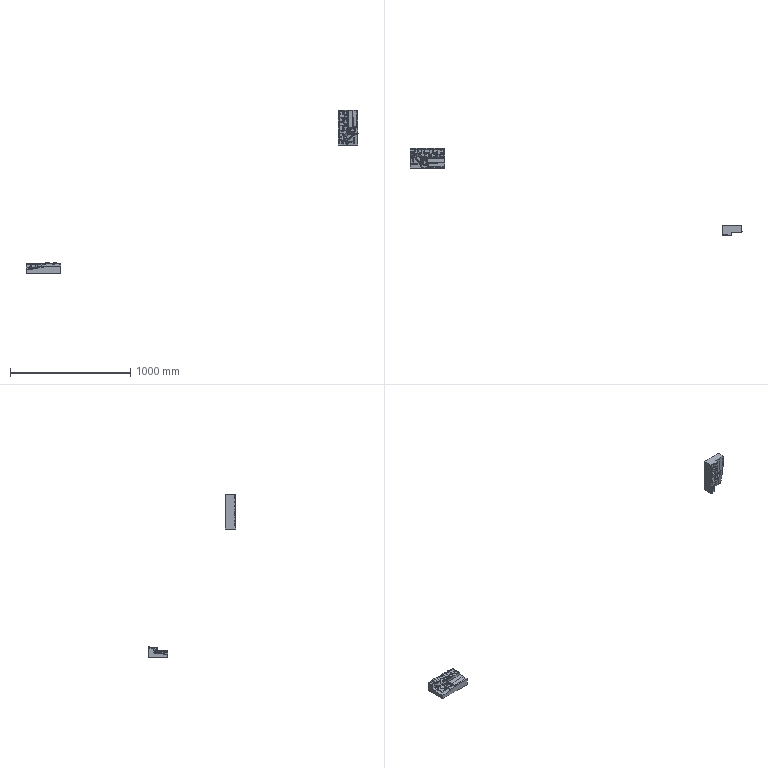NC program | NX | posted with a generic post | part box 2756 x 729.572 x 1353 mm
Lines 40259 to 41352 of 54396:
(CAVITY_MILL_1_COPY_COPY , TOOL : D6R3)
N80504 M6
N80506 G54
N80508 G17 G0 G90 X-104.537 Y-0.08 B0. C0. S3000 M3
N80510 G43 Z97. H0
N80512 Z88.216
N80514 G94 G1 Z88.016 F2500.
N80516 X-101.653 Y0.312
N80518 X-98.238 Y0.776
N80520 X-97.634 Y0.793
N80522 G2 X-96.274 Y0.137 R1.531
N80524 G1 X-96.255 Y-0.466
N80526 X-96.271 Y-7.828
N80528 G2 X-96.837 Y-8.503 R0.687
N80530 G1 X-97.634 Y-8.646
N80532 X-101.51 Y-8.335
N80534 X-104.477 Y-8.097
N80536 Z88.216
N80538 G0 Z89.3
N80540 X-104.765 Y2.482
N80542 Z88.019
N80544 G1 Z87.819
N80546 X-104.68 Y0.984
N80548 X-101.685 Y1.154
N80550 X-98.008 Y1.363
N80552 G2 X-95.577 Y0.741 R4.145
N80554 G1 X-95.179 Y0.137
N80556 X-95.167 Y-0.466
N80558 X-95.165 Y-7.707
N80560 X-95.217 Y-8.141
N80562 G2 X-97.029 Y-9.164 R2.101
N80564 X-101.54 Y-9.093 R116.617
N80566 G1 X-104.539 Y-8.987
N80568 X-104.627 Y-10.446
N80570 Z88.019
N80572 G0 Z88.316
N80574 X-104.659 Y3.
N80576 Z87.823
N80578 G1 Z87.623
N80580 X-104.604 Y1.515
N80582 X-101.605 Y1.598
N80584 G2 X-97.634 Y1.684 R323.824
N80586 X-95.101 Y1.023 R4.533
N80588 X-94.83 Y0.807 R1.373
N80590 G1 X-92.945 Y-1.138
N80592 Z87.823
N80594 G0 Z88.513
N80596 X-104.282 Y3.348
N80598 Z87.626
N80600 G1 Z87.426
N80602 X-104.24 Y1.858
N80604 X-101.24 Y1.924
N80606 G2 X-97.634 Y1.989 R469.677
N80608 X-95.269 Y1.542 R6.532
N80610 G1 X-92.399 Y0.42
N80612 Z87.626
N80614 G0 Z88.623
N80616 X-104.188 Y3.801
N80618 Z87.232
N80620 G1 Z87.032
N80622 X-104.165 Y2.309
N80624 X-101.166 Y2.34
N80626 G2 X-97.029 Y2.369 R617.615
N80628 X-95.492 Y2.165 R6.148
N80630 G1 X-91.675 Y1.158
N80632 Z87.232
N80634 G0 Z88.819
N80636 X-92.958 Y-6.801
N80638 Z87.823
N80640 G1 Z87.623
N80642 X-94.825 Y-8.656
N80644 G2 X-97.029 Y-9.572 R3.15
N80646 X-101.464 Y-9.517 R222.575
N80648 G1 X-104.463 Y-9.451
N80650 X-104.516 Y-10.93
N80652 Z87.823
N80654 G0 Z88.119
N80656 X-92.406 Y-8.315
N80658 Z87.626
N80660 G1 Z87.426
N80662 X-95.307 Y-9.458
N80664 G2 X-97.634 Y-9.884 R6.116
N80666 X-101.119 Y-9.818 R522.737
N80668 G1 X-104.118 Y-9.751
N80670 X-104.16 Y-11.242
N80672 Z87.626
N80674 G0 Z88.623
N80676 X-91.679 Y-9.046
N80678 Z87.232
N80680 G1 Z87.032
N80682 X-95.472 Y-10.039
N80684 G2 X-97.634 Y-10.285 R7.65
N80686 X-101.025 Y-10.243 R973.582
N80688 G1 X-104.025 Y-10.201
N80690 X-104.051 Y-11.696
N80692 Z87.232
N80694 G0 Z88.426
N80696 X-93.828 Y-12.541
N80698 Z81.723
N80700 G1 Z81.523
N80702 X-93.829 Y-11.041
N80704 X-96.829 Y-11.042
N80706 X-97.47 Y-11.043
N80708 X-97.577 Y-11.032
N80710 X-97.65 Y-11.111
N80712 X-97.651 Y-13.112
N80714 X-97.652 Y-16.112
N80716 X-96.152 Y-16.113
N80718 Z81.723
N80720 G0 Z87.332
N80722 X-93.009 Y-12.543
N80724 Z81.526
N80726 G1 Z81.326
N80728 X-93.02 Y-11.053
N80730 X-96.02
N80732 G2 X-96.863 Y-11.053 R436.94
N80734 G1 X-96.937 Y-11.328
N80736 X-96.933 Y-13.151
N80738 X-96.928 Y-16.151
N80740 X-95.428 Y-16.149
N80742 Z81.526
N80744 G0 Z81.823
N80746 X-92.425 Y-12.534
N80748 Z81.329
N80750 G1 Z81.129
N80752 X-92.43 Y-11.034
N80754 X-95.43 Y-11.043
N80756 X-96.327 Y-11.046
N80758 X-96.385 Y-11.03
N80760 X-96.408 Y-11.086
N80762 X-96.404 Y-13.199
N80764 X-96.398 Y-16.199
N80766 X-94.898 Y-16.196
N80768 Z81.329
N80770 G0 Z81.626
N80772 X-91.939 Y-12.536
N80774 Z81.132
N80776 G1 Z80.932
N80778 Y-11.035
N80780 X-94.939 Y-11.039
N80782 X-95.86 Y-11.041
N80784 X-95.945 Y-11.026
N80786 X-95.999 Y-11.093
N80788 X-95.991 Y-13.181
N80790 X-95.978 Y-16.181
N80792 X-94.478 Y-16.175
N80794 Z81.132
N80796 G0 Z81.429
N80798 X-91.542 Y-12.536
N80800 Z80.936
N80802 G1 Z80.736
N80804 X-91.543 Y-11.031
N80806 X-94.543 Y-11.043
N80808 X-95.589 Y-11.047
N80810 X-95.643 Y-11.044
N80812 X-95.64 Y-11.099
N80814 X-95.631 Y-13.282
N80816 X-95.619 Y-16.282
N80818 X-94.119 Y-16.276
N80820 Z80.936
N80822 G0 Z81.232
N80824 X-91.155 Y-12.542
N80826 Z80.739
N80828 G1 Z80.539
N80830 Y-11.042
N80832 X-94.155
N80834 X-95.217
N80836 X-95.28 Y-11.051
N80838 X-95.316 Y-11.081
N80840 X-95.306 Y-13.26
N80842 X-95.293 Y-16.26
N80844 X-93.793 Y-16.254
N80846 Z80.739
N80848 G0 Z81.036
N80850 X-90.816 Y-12.531
N80852 Z80.542
N80854 G1 Z80.342
N80856 Y-11.03
N80858 X-93.816 Y-11.04
N80860 X-95.013 Y-11.044
N80862 X-95.044 Y-11.078
N80864 X-95.034 Y-13.323
N80866 X-95.02 Y-16.323
N80868 X-93.52 Y-16.317
N80870 Z80.542
N80872 G0 Z80.839
N80874 X-90.462 Y-12.536
N80876 Z80.345
N80878 G1 Z80.145
N80880 Y-11.031
N80882 X-93.462 Y-11.038
N80884 X-94.73 Y-11.041
N80886 X-94.787 Y-11.03
N80888 X-94.79 Y-11.088
N80890 X-94.777 Y-13.407
N80892 X-94.761 Y-16.407
N80894 X-93.261 Y-16.398
N80896 Z80.345
N80898 G0 Z80.642
N80900 X-90.187 Y-12.536
N80902 Z80.148
N80904 G1 Z79.948
N80906 X-90.188 Y-11.024
N80908 X-93.188 Y-11.038
N80910 X-94.53 Y-11.045
N80912 X-94.544 Y-11.063
N80914 X-94.534 Y-13.232
N80916 X-94.52 Y-16.232
N80918 X-93.02 Y-16.225
N80920 Z80.148
N80922 G0 Z80.445
N80924 X-89.916 Y-12.531
N80926 Z79.952
N80928 G1 Z79.752
N80930 Y-11.027
N80932 X-92.916 Y-11.038
N80934 X-94.331 Y-11.044
N80936 X-94.342 Y-11.067
N80938 X-94.331 Y-13.294
N80940 X-94.315 Y-16.294
N80942 X-92.815 Y-16.287
N80944 Z79.952
N80946 G0 Z80.248
N80948 X-89.657 Y-12.536
N80950 Z79.755
N80952 G1 Z79.555
N80954 Y-11.036
N80956 X-92.657
N80958 X-92.8
N80960 X-94.1 Y-11.042
N80962 X-94.143 Y-11.127
N80964 X-94.13 Y-13.358
N80966 X-94.113 Y-16.358
N80968 X-92.613 Y-16.349
N80970 Z79.755
N80972 G0 Z80.052
N80974 X-89.455 Y-12.536
N80976 Z79.558
N80978 G1 Z79.358
N80980 Y-11.036
N80982 X-92.455
N80984 X-92.8
N80986 X-93.932 Y-11.044
N80988 X-93.944 Y-11.055
N80990 X-93.956 Y-11.127
N80992 X-93.945 Y-13.339
N80994 X-93.931 Y-16.339
N80996 X-92.431 Y-16.332
N80998 Z79.558
N81000 G0 Z79.855
N81002 X-89.203 Y-12.536
N81004 Z79.361
N81006 G1 Z79.161
N81008 Y-11.036
N81010 X-92.203
N81012 X-92.8
N81014 X-93.763 Y-11.043
N81016 X-93.801 Y-11.127
N81018 X-93.79 Y-13.391
N81020 X-93.774 Y-16.391
N81022 X-92.274 Y-16.383
N81024 Z79.361
N81026 G0 Z79.658
N81028 X-88.975 Y-12.536
N81030 Z79.165
N81032 G1 Z78.965
N81034 Y-11.036
N81036 X-91.975
N81038 X-92.8
N81040 X-93.614 Y-11.042
N81042 X-93.647 Y-11.127
N81044 X-93.634 Y-13.536
N81046 X-93.617 Y-16.536
N81048 X-92.117 Y-16.527
N81050 Z79.165
N81052 G0 Z79.461
N81054 X-88.773 Y-12.531
N81056 Z78.968
N81058 G1 Z78.768
N81060 Y-11.024
N81062 X-91.773 Y-11.034
N81064 X-93.425 Y-11.039
N81066 X-93.494 Y-11.038
N81068 X-93.493 Y-11.107
N81070 X-93.479 Y-13.46
N81072 X-93.462 Y-16.46
N81074 X-91.962 Y-16.452
N81076 Z78.968
N81078 G0 Z79.265
N81080 X-88.605 Y-12.536
N81082 Z78.771
N81084 G1 Z78.571
N81086 Y-11.036
N81088 X-91.605
N81090 X-92.8
N81092 X-93.345 Y-11.043
N81094 X-93.349 Y-11.127
N81096 X-93.336 Y-13.439
N81098 X-93.319 Y-16.439
N81100 X-91.819 Y-16.431
N81102 Z78.771
N81104 G0 Z79.068
N81106 X-88.437 Y-12.536
N81108 Z78.574
N81110 G1 Z78.374
N81112 X-88.438 Y-11.036
N81114 X-91.438
N81116 X-92.8
N81118 X-93.204 Y-11.042
N81120 X-93.221 Y-11.328
N81122 X-93.207 Y-13.49
N81124 X-93.186 Y-16.49
N81126 X-91.686 Y-16.48
N81128 Z78.574
N81130 G0 Z78.871
N81132 X-88.212 Y-12.536
N81134 Z78.377
N81136 G1 Z78.177
N81138 Y-11.036
N81140 X-91.212
N81142 X-92.8 Y-11.037
N81144 X-93.071 Y-11.041
N81146 X-93.085 Y-11.127
N81148 X-93.065 Y-13.542
N81150 X-93.039 Y-16.542
N81152 X-91.539 Y-16.529
N81154 Z78.377
N81156 G0 Z78.674
N81158 X-87.981 Y-12.531
N81160 Z78.181
N81162 G1 Z77.981
N81164 Y-11.022
N81166 X-90.981 Y-11.031
N81168 X-92.881 Y-11.037
N81170 X-92.916 Y-11.035
N81172 X-92.914 Y-11.07
N81174 X-92.884 Y-13.709
N81176 X-92.851 Y-16.709
N81178 X-91.351 Y-16.693
N81180 Z78.181
N81182 G0 Z78.477
N81184 X-87.486 Y-12.534
N81186 Z77.984
N81188 G1 Z77.784
N81190 Y-11.034
N81192 X-90.486
N81194 X-92.195
N81196 X-92.683 Y-11.048
N81198 X-92.72 Y-11.328
N81200 X-92.673 Y-14.112
N81202 X-92.623 Y-17.111
N81204 X-91.123 Y-17.086
N81206 Z77.984
N81208 G0 Z78.281
N81210 X-86.689 Y-12.531
N81212 Z77.787
N81214 G1 Z77.587
N81216 Y-11.031
N81218 X-89.689
N81220 X-90.987
N81222 X-92.328 Y-11.035
N81224 X-92.394 Y-11.018
N81226 X-92.429 Y-11.077
N81228 G3 X-92.394 Y-14.85 R446.531
N81230 G1 X-92.355 Y-17.849
N81232 X-90.845 Y-17.819
N81234 Z77.787
N81236 G0 Z83.31
N81238 X-30.322 Y-12.532
N81240 Z82.313
N81242 G1 Z82.113
N81244 X-30.323 Y-11.032
N81246 X-33.323 Y-11.035
N81248 X-33.582 Y-11.036
N81250 X-34.041 Y-11.067
N81252 X-34.116 Y-11.082
N81254 X-34.123 Y-12.958
N81256 X-34.136 Y-15.958
N81258 X-32.636 Y-15.964
N81260 Z82.313
N81262 G0 Z82.61
N81264 X-29.431 Y-12.536
N81266 Z82.116
N81268 G1 Z81.916
N81270 X-29.432 Y-11.036
N81272 X-32.432 Y-11.039
N81274 X-33.198
N81276 X-33.281 Y-11.032
N81278 X-33.315 Y-11.108
N81280 X-33.318 Y-12.955
N81282 X-33.323 Y-15.955
N81284 X-31.823 Y-15.958
N81286 Z82.116
N81288 G0 Z82.413
N81290 X-28.773 Y-12.528
N81292 Z81.919
N81294 G1 Z81.719
N81296 X-28.777 Y-11.036
N81298 X-31.777
N81300 X-32.374
N81302 X-32.689 Y-11.051
N81304 X-32.755 Y-11.082
N81306 X-32.756 Y-13.31
N81308 X-32.758 Y-16.31
N81310 X-31.258 Y-16.311
N81312 Z81.919
N81314 G0 Z82.216
N81316 X-28.286 Y-12.529
N81318 Z81.723
N81320 G1 Z81.523
N81322 X-28.29 Y-11.029
N81324 X-31.29 Y-11.036
N81326 X-31.852 Y-11.038
N81328 X-32.239 Y-11.047
N81330 X-32.303 Y-11.085
N81332 X-32.304 Y-13.189
N81334 Y-16.189
N81336 X-30.804
N81338 Z81.723
N81340 G0 Z82.019
N81342 X-27.839 Y-12.534
N81344 Z81.526
N81346 G1 Z81.326
N81348 X-27.85 Y-11.035
N81350 X-30.85 Y-11.036
N81352 X-31.852 Y-11.037
N81354 X-31.935 Y-11.089
N81356 X-31.934 Y-13.232
N81358 X-31.933 Y-16.232
N81360 X-30.433
N81362 Z81.526
N81364 G0 Z81.823
N81366 X-27.453 Y-12.527
N81368 Z81.329
N81370 G1 Z81.129
N81372 X-27.47 Y-11.046
N81374 X-30.47 Y-11.043
N81376 G2 X-31.553 Y-11.039 R239.955
N81378 G1 X-31.596 Y-11.068
N81380 X-31.609 Y-11.127
N81382 X-31.608 Y-13.323
N81384 X-31.606 Y-16.323
N81386 X-30.106
N81388 Z81.329
N81390 G0 Z81.626
N81392 X-27.096 Y-12.521
N81394 Z81.132
N81396 G1 Z80.932
N81398 X-27.101 Y-11.021
N81400 X-30.101 Y-11.031
N81402 X-31.246 Y-11.035
N81404 X-31.318
N81406 Y-11.107
N81408 X-31.317 Y-13.279
N81410 X-31.315 Y-16.279
N81412 X-29.815
N81414 Z81.132
N81416 G0 Z81.429
N81418 X-26.8 Y-12.525
N81420 Z80.936
N81422 G1 Z80.736
N81424 X-26.804 Y-11.025
N81426 X-29.804 Y-11.033
N81428 X-30.561 Y-11.034
N81430 X-31.031 Y-11.043
N81432 X-31.053 Y-11.065
N81434 X-31.051 Y-13.377
N81436 X-31.05 Y-16.377
N81438 X-29.55 Y-16.376
N81440 Z80.936
N81442 G0 Z81.232
N81444 X-26.479 Y-12.534
N81446 Z80.739
N81448 G1 Z80.539
N81450 X-26.481 Y-11.034
N81452 X-29.481 Y-11.037
N81454 X-30.796 Y-11.039
N81456 X-30.819 Y-11.062
N81458 X-30.817 Y-13.286
N81460 X-30.815 Y-16.286
N81462 X-29.315 Y-16.284
N81464 Z80.739
N81466 G0 Z81.036
N81468 X-26.203 Y-12.53
N81470 Z80.542
N81472 G1 Z80.342
N81474 X-26.204 Y-11.025
N81476 X-29.204 Y-11.032
N81478 X-29.957 Y-11.034
N81480 X-30.561 Y-11.044
N81482 X-30.586 Y-11.06
N81484 X-30.584 Y-13.181
N81486 X-30.581 Y-16.181
N81488 X-29.081 Y-16.18
N81490 Z80.542
N81492 G0 Z80.839
N81494 X-27.435 Y-12.53
N81496 Z80.345
N81498 G1 Z80.145
N81500 Y-11.021
N81502 X-28.935 Y-11.032
N81504 X-30.362 Y-11.043
N81506 X-30.401 Y-11.127
N81508 X-30.398 Y-13.339
N81510 X-30.395 Y-16.339
N81512 X-28.895 Y-16.337
N81514 Z80.345
N81516 G0 Z80.642
N81518 X-27.225 Y-12.53
N81520 Z80.148
N81522 G1 Z79.948
N81524 X-27.226 Y-11.023
N81526 X-28.726 Y-11.031
N81528 X-30.17 Y-11.039
N81530 X-30.179 Y-11.044
N81532 X-30.22 Y-11.127
N81534 X-30.217 Y-13.432
N81536 X-30.213 Y-16.432
N81538 X-28.713 Y-16.43
N81540 Z80.148
N81542 G0 Z80.445
N81544 X-25.488 Y-12.526
N81546 Z79.952
N81548 G1 Z79.752
N81550 X-25.489 Y-11.022
N81552 X-28.489 Y-11.03
N81554 X-29.973 Y-11.035
N81556 X-30.041 Y-11.033
N81558 X-30.04 Y-11.102
N81560 X-30.036 Y-13.342
N81562 X-30.032 Y-16.342
N81564 X-28.532 Y-16.34
N81566 Z79.952
N81568 G0 Z80.248
N81570 X-25.248 Y-12.53
N81572 Z79.755
N81574 G1 Z79.555
N81576 X-25.249 Y-11.03
N81578 X-28.249 Y-11.031
N81580 X-28.748
N81582 X-29.852 Y-11.039
N81584 X-29.865 Y-11.05
N81586 X-29.876 Y-11.328
N81588 X-29.873 Y-13.336
N81590 X-29.869 Y-16.336
N81592 X-28.369 Y-16.334
N81594 Z79.755
N81596 G0 Z80.052
N81598 X-25.045 Y-12.53
N81600 Z79.558
N81602 G1 Z79.358
N81604 X-25.046 Y-11.03
N81606 X-28.046 Y-11.031
N81608 X-28.748
N81610 X-29.703 Y-11.038
N81612 X-29.717 Y-11.056
N81614 X-29.714 Y-13.327
N81616 X-29.711 Y-16.327
N81618 X-28.211 Y-16.326
N81620 Z79.558
N81622 G0 Z79.855
N81624 X-24.849 Y-12.526
N81626 Z79.361
N81628 G1 Z79.161
N81630 X-24.85 Y-11.017
N81632 X-27.85 Y-11.03
N81634 X-29.573 Y-11.037
N81636 X-29.584 Y-11.061
N81638 X-29.582 Y-13.276
N81640 X-29.578 Y-16.276
N81642 X-28.078 Y-16.275
N81644 Z79.361
N81646 G0 Z79.658
N81648 X-24.686 Y-12.526
N81650 Z79.165
N81652 G1 Z78.965
N81654 Y-11.018
N81656 X-27.686 Y-11.029
N81658 X-29.432 Y-11.035
N81660 X-29.465 Y-11.127
N81662 X-29.462 Y-13.288
N81664 X-29.458 Y-16.288
N81666 X-27.958 Y-16.285
N81668 Z79.165
N81670 G0 Z79.461
N81672 X-24.549 Y-12.529
N81674 Z78.968
N81676 G1 Z78.768
N81678 Y-11.029
N81680 X-27.549 Y-11.031
N81682 X-28.748
N81684 X-29.34 Y-11.038
N81686 X-29.337 Y-13.273
N81688 X-29.333 Y-16.273
N81690 X-27.833 Y-16.271
N81692 Z78.968
N81694 G0 Z79.265
N81696 X-24.417 Y-12.529
N81698 Z78.771
N81700 G1 Z78.571
N81702 Y-11.029
N81704 X-27.417 Y-11.031
N81706 X-28.748
N81708 X-29.229 Y-11.037
N81710 X-29.234 Y-11.127
N81712 X-29.23 Y-13.397
N81714 X-29.224 Y-16.397
N81716 X-27.724 Y-16.394
N81718 Z78.771
N81720 G0 Z79.068
N81722 X-24.298 Y-12.526
N81724 Z78.574
N81726 G1 Z78.374
N81728 Y-11.014
N81730 X-27.298 Y-11.028
N81732 X-29.109 Y-11.037
N81734 X-29.118 Y-11.061
N81736 X-29.129 Y-11.328
N81738 X-29.123 Y-13.478
N81740 X-29.116 Y-16.478
N81742 X-27.616 Y-16.474
N81744 Z78.574
N81746 G0 Z78.871
N81748 X-24.186 Y-12.526
N81750 Z78.377
N81752 G1 Z78.177
N81754 Y-11.014
N81756 X-27.186 Y-11.027
N81758 X-28.998 Y-11.036
N81760 X-29.012 Y-11.328
N81762 X-29.003 Y-13.421
N81764 X-28.989 Y-16.421
N81766 X-27.489 Y-16.415
N81768 Z78.377
N81770 G0 Z78.674
N81772 X-24.009 Y-12.526
N81774 Z78.181
N81776 G1 Z77.981
N81778 X-24.01 Y-11.013
N81780 X-27.01 Y-11.027
N81782 X-28.848 Y-11.035
N81784 X-28.867 Y-11.065
N81786 X-28.854 Y-13.564
N81788 X-28.838 Y-16.564
N81790 X-27.338 Y-16.556
N81792 Z78.181
N81794 G0 Z78.477
N81796 X-23.768 Y-12.528
N81798 Z77.984
N81800 G1 Z77.784
N81802 X-23.769 Y-11.028
N81804 X-26.769 Y-11.029
N81806 X-28.144 Y-11.03
N81808 X-28.674 Y-11.039
N81810 X-28.714 Y-11.127
N81812 X-28.686 Y-13.848
N81814 X-28.655 Y-16.848
N81816 X-27.155 Y-16.832
N81818 Z77.984
N81820 G0 Z78.281
N81822 X-23.276 Y-12.528
N81824 Z77.787
N81826 G1 Z77.587
N81828 Y-11.028
N81830 X-26.276 Y-11.029
N81832 X-28.144 Y-11.03
N81834 X-28.454 Y-11.042
N81836 X-28.476 Y-11.076
N81838 X-28.488 Y-11.328
N81840 X-28.459 Y-14.227
N81842 X-28.429 Y-17.226
N81844 X-26.916 Y-17.199
N81846 Z77.787
N81848 G0 Z78.084
N81850 X-22.435 Y-12.525
N81852 Z77.59
N81854 G1 Z77.39
N81856 Y-11.025
N81858 X-25.435 Y-11.026
N81860 X-26.935
N81862 X-28.028 Y-11.032
N81864 X-28.172 Y-11.08
N81866 X-28.184 Y-11.099
N81868 X-28.079 Y-14.663
N81870 X-27.991 Y-17.661
N81872 X-26.492 Y-17.617
N81874 Z77.59
N81876 G0 Z77.887
N81878 X-22.353 Y-15.644
N81880 Z77.394
N81882 G1 Z77.194
N81884 X-23.604 Y-14.313
N81886 X-23.872 Y-14.027
N81888 X-23.508
N81890 G2 X-21.114 Y-11.026 R6.06
N81892 G1 X-25.727 Y-11.028
N81894 X-26.935 Y-11.035
N81896 X-27.54 Y-11.081
N81898 X-27.639 Y-11.127
N81900 G3 X-26.935 Y-15.149 R13.365
N81902 G1 X-22.828 Y-19.519
N81904 X-20.773 Y-21.705
N81906 X-19.68 Y-20.678
N81908 Z77.394
N81910 G0 Z79.571
N81912 X-27.575 Y-32.254
N81914 Z78.574
N81916 G1 Z78.374
N81918 X-29.075 Y-32.258
N81920 X-29.068 Y-35.258
N81922 X-29.067 Y-35.465
N81924 G3 X-26.331 Y-38.268 R2.752
N81926 G1 X-26.095
N81928 X-23.095 Y-38.272
N81930 X-23.094 Y-36.772
N81932 Z78.574
N81934 G0 Z78.871
N81936 X-27.419 Y-32.008
N81938 Z78.377
N81940 G1 Z78.177
N81942 X-28.919 Y-32.014
N81944 X-28.905 Y-35.014
N81946 X-28.903 Y-35.465
N81948 G3 X-26.331 Y-38.12 R2.6
N81950 G1 X-25.786 Y-38.121
N81952 X-22.786 Y-38.13
N81954 X-22.782 Y-36.63
N81956 Z78.377
N81958 G0 Z78.674
N81960 X-27.257 Y-31.525
N81962 Z78.181
N81964 G1 Z77.981
N81966 X-28.765 Y-31.533
N81968 X-28.734 Y-34.533
N81970 X-28.725 Y-35.465
N81972 G3 X-26.331 Y-37.928 R2.435
N81974 G1 X-25.366 Y-37.933
N81976 X-22.366 Y-37.95
N81978 X-22.358 Y-36.45
N81980 Z78.181
N81982 G0 Z78.477
N81984 X-27.008 Y-31.026
N81986 Z77.984
N81988 G1 Z77.784
N81990 X-28.508 Y-31.042
N81992 X-28.477 Y-34.042
N81994 X-28.461 Y-35.528
N81996 G3 X-26.33 Y-37.665 R2.16
N81998 X-24.849 Y-37.684 R3110.17
N82000 G1 X-21.849 Y-37.721
N82002 X-21.832 Y-36.22
N82004 Z77.984
N82006 G0 Z78.281
N82008 X-26.656 Y-31.774
N82010 Z77.787
N82012 G1 Z77.587
N82014 X-28.168 Y-31.801
N82016 X-28.113 Y-33.3
N82018 X-28.03 Y-35.564
N82020 G3 X-26.299 Y-37.277 R1.779
N82022 X-24.057 Y-37.333 R1197.162
N82024 G1 X-21.058 Y-37.405
N82026 X-21.026 Y-35.901
N82028 Z77.787
N82030 G0 Z83.31
N82032 X-16.902 Y-42.938
N82034 Z82.313
N82036 G1 Z82.113
N82038 X-16.754 Y-44.67
N82040 X-16.612 Y-46.326
N82042 Y-46.552
N82044 G3 X-16.059 Y-46.647 R0.499
N82046 X-14.54 Y-46.997 R12.565
N82048 G1 X-13.995 Y-45.562
N82050 Z82.313
N82052 G0 Z85.671
N82054 X-15.683 Y-76.069
N82056 Z82.313
N82058 G1 Z82.113
N82060 X-15.736 Y-74.572
N82062 X-18.734 Y-74.658
N82064 X-19.761 Y-74.687
N82066 X-21.658 Y-75.222
N82068 X-21.748 Y-75.291
N82070 G2 X-21.856 Y-77.15 R4.812
N82072 G1 X-22.3 Y-78.863
N82074 Z82.313
N82076 G0 Z85.474
N82078 X-45.61 Y-61.672
N82080 Z82.116
N82082 G1 Z81.916
N82084 X-44.11
N82086 Y-58.672
N82088 Y-57.047
N82090 G3 X-44.876 Y-56.101 R1.962
N82092 X-46.001 Y-55.414 R25.31
N82094 G1 X-46.868 Y-56.646
N82096 Z82.116
N82098 G0 Z82.413
N82100 X-46.879 Y-61.943
N82102 Z81.919
N82104 G1 Z81.719
N82106 X-45.379
N82108 Y-58.943
N82110 Y-57.047
N82112 G3 X-46.182 Y-56.147 R1.641
N82114 X-47.479 Y-55.52 R47.482
N82116 G1 X-48.264 Y-56.809
N82118 Z81.919
N82120 G0 Z82.216
N82122 X-48.148 Y-62.061
N82124 Z81.723
N82126 G1 Z81.523
N82128 X-46.648
N82130 Y-59.061
N82132 Y-57.047
N82134 G3 X-47.607 Y-56.108 R1.894
N82136 X-48.797 Y-55.602 R58.771
N82138 G1 X-49.55 Y-56.915
N82140 Z81.723
N82142 G0 Z82.019
N82144 X-49.418 Y-62.121
N82146 Z81.526
N82148 G1 Z81.326
N82150 X-47.918
N82152 Y-59.121
N82154 Y-57.047
N82156 X-48.175 Y-56.585
N82158 X-48.689 Y-56.287
N82160 G3 X-50.032 Y-55.687 R37.569
N82162 G1 X-50.795 Y-56.993
N82164 Z81.526
N82166 G0 Z81.823
N82168 X-50.687 Y-62.131
N82170 Z81.329
N82172 G1 Z81.129
N82174 X-49.187
N82176 Y-59.131
N82178 Y-57.047
N82180 X-49.45 Y-56.585
N82182 G3 X-51.382 Y-55.642 R13.924
N82184 G1 X-52.107 Y-56.969
N82186 Z81.329
N82188 G0 Z81.626
N82190 X-51.956 Y-62.138
N82192 Z81.132
N82194 G1 Z80.932
N82196 X-50.456
N82198 Y-59.138
N82200 Y-57.05
N82202 X-50.724 Y-56.585
N82204 G3 X-52.618 Y-55.67 R13.194
N82206 G1 X-53.353 Y-56.995
N82208 Z81.132
N82210 G0 Z81.429
N82212 X-53.225 Y-62.138
N82214 Z80.936
N82216 G1 Z80.736
N82218 X-51.725
N82220 Y-59.138
N82222 Y-57.057
N82224 X-51.998 Y-56.585
N82226 G3 X-53.845 Y-55.7 R6.384
N82228 G1 X-55.284 Y-55.277
N82230 X-55.709 Y-56.711
N82232 Z80.936
N82234 G0 Z81.232
N82236 X-54.494 Y-62.14
N82238 Z80.739
N82240 G1 Z80.539
N82242 X-52.994
N82244 Y-59.14
N82246 Y-57.086
N82248 X-53.268 Y-56.585
N82250 G3 X-55.075 Y-55.731 R13.963
N82252 G1 X-55.825 Y-57.051
N82254 Z80.739
N82256 G0 Z81.036
N82258 X-55.764 Y-62.14
N82260 Z80.542
N82262 G1 Z80.342
N82264 X-54.264
N82266 Y-59.14
N82268 Y-57.113
N82270 X-54.537 Y-56.585
N82272 G3 X-55.94 Y-55.873 R4.079
N82274 G1 X-56.302 Y-55.764
N82276 X-57.737 Y-55.328
N82278 X-58.166 Y-56.768
N82280 Z80.542
N82282 G0 Z83.113
N82284 X-67.755 Y-37.078
N82286 Z78.771
N82288 G1 Z78.571
N82290 X-67.744 Y-38.576
N82292 X-64.745 Y-38.559
N82294 G2 X-64.428 Y-38.557 R2376.602
N82296 G3 X-61.723 Y-35.877 R2.721
N82298 G1 X-61.717 Y-35.504
N82300 X-61.673 Y-32.504
N82302 X-63.174 Y-32.487
N82304 Z78.771
N82306 G0 Z79.068
N82308 X-68.108 Y-36.94
N82310 Z78.574
N82312 G1 Z78.374
N82314 X-68.093 Y-38.44
N82316 X-65.093 Y-38.41
N82318 X-64.428 Y-38.403
N82320 G3 X-61.895 Y-35.931 R2.561
N82322 G1 X-61.879 Y-35.465
N82324 X-61.876 Y-35.275
N82326 X-61.836 Y-32.275
N82328 X-63.335 Y-32.255
N82330 Z78.574
N82332 G0 Z78.871
N82334 X-68.497 Y-36.732
N82336 Z78.377
N82338 G1 Z78.177
N82340 X-68.484 Y-38.229
N82342 X-65.484 Y-38.209
N82344 G2 X-64.438 Y-38.202 R2288.528
N82346 G3 X-62.08 Y-35.878 R2.373
N82348 G1 X-62.058 Y-34.823
N82350 X-61.996 Y-31.824
N82352 X-63.496 Y-31.792
N82354 Z78.377
N82356 G0 Z78.674
N82358 X-69.151 Y-36.483
N82360 Z78.181
N82362 G1 Z77.981
N82364 X-69.132 Y-37.982
N82366 X-66.132 Y-37.944
N82368 X-64.448 Y-37.922
N82370 G3 X-62.344 Y-35.831 R2.132
N82372 G1 X-62.313 Y-34.255
N82374 X-62.255 Y-31.256
N82376 X-63.754 Y-31.227
N82378 Z78.181
N82380 G0 Z78.477
N82382 X-69.792 Y-36.031
N82384 Z77.984
N82386 G1 Z77.784
N82388 X-69.771 Y-37.529
N82390 X-66.772 Y-37.492
N82392 G2 X-64.473 Y-37.465 R2016.532
N82394 G3 X-62.771 Y-35.79 R1.722
N82396 G1 X-62.713 Y-33.676
N82398 X-62.63 Y-30.677
N82400 X-64.13 Y-30.636
N82402 Z77.984
N82404 G0 Z78.281
N82406 X-70.293 Y-27.863
N82408 Z77.787
N82410 G1 Z77.587
N82412 X-70.143 Y-29.355
N82414 X-67.158 Y-29.055
N82416 X-63.693 Y-28.706
N82418 G3 X-63.307 Y-27.62 R2.228
N82420 X-63.139 Y-25.849 R178.287
N82422 G1 X-63.004 Y-24.355
N82424 X-64.505 Y-24.233
N82426 Z77.787
N82428 G0 Z83.31
N82430 X-57.795 Y-15.453
N82432 Z82.313
N82434 G1 Z82.113
N82436 X-56.295 Y-15.457
N82438 X-56.288 Y-12.457
N82440 X-56.285 Y-11.328
N82442 X-56.318 Y-11.089
N82444 G3 X-56.955 Y-11.049 R10.142
N82446 G1 X-57.85 Y-12.542
N82448 Z82.313
N82450 G0 Z82.61
N82452 X-58.77 Y-16.121
N82454 Z82.116
N82456 G1 Z81.916
N82458 X-57.27 Y-16.131
N82460 X-57.25 Y-13.131
N82462 X-57.246 Y-12.535
N82464 X-57.235 Y-11.115
N82466 X-57.296 Y-11.034
N82468 X-57.397 Y-11.042
N82470 X-58.083 Y-11.041
N82472 X-61.083 Y-11.036
N82474 X-61.086 Y-12.536
N82476 Z82.116
N82478 G0 Z82.413
N82480 X-59.369 Y-16.305
N82482 Z81.919
N82484 G1 Z81.719
N82486 X-57.869 Y-16.317
N82488 X-57.844 Y-13.318
N82490 X-57.825 Y-11.079
N82492 X-57.907 Y-11.039
N82494 X-58.839 Y-11.038
N82496 X-61.839 Y-11.033
N82498 X-61.841 Y-12.533
N82500 Z81.919
N82502 G0 Z82.216
N82504 X-59.837 Y-16.325
N82506 Z81.723
N82508 G1 Z81.523
N82510 X-58.337 Y-16.339
N82512 X-58.309 Y-13.339
N82514 X-58.297 Y-11.931
N82516 X-58.288 Y-11.08
N82518 X-58.357 Y-11.051
N82520 X-58.665 Y-11.042
N82522 X-59.323 Y-11.041
N82524 X-62.323 Y-11.033
N82526 X-62.327 Y-12.533
N82528 Z81.723
N82530 G0 Z82.019
N82532 X-60.217 Y-16.316
N82534 Z81.526
N82536 G1 Z81.326
N82538 X-58.717 Y-16.332
N82540 X-58.686 Y-13.332
N82542 X-58.664 Y-11.089
N82544 X-58.715 Y-11.023
N82546 X-58.798 Y-11.038
N82548 G2 X-59.801 Y-11.044 R246.17
N82550 G1 X-62.801 Y-11.058
N82552 X-62.812 Y-12.54
N82554 Z81.526
N82556 G0 Z81.823
N82558 X-60.564 Y-16.369
N82560 Z81.329
N82562 G1 Z81.129
N82564 X-59.064 Y-16.382
N82566 X-59.036 Y-13.382
N82568 X-59.016 Y-11.079
N82570 X-59.065 Y-11.042
N82572 G3 X-60.199 Y-11.037 R3776.671
N82574 G1 X-63.199 Y-11.022
N82576 X-63.205 Y-12.523
N82578 Z81.329
N82580 G0 Z81.626
N82582 X-60.854 Y-16.337
N82584 Z81.132
N82586 G1 Z80.932
N82588 X-59.354 Y-16.352
N82590 X-59.324 Y-13.352
N82592 X-59.301 Y-11.085
N82594 X-59.311 Y-11.026
N82596 X-59.37 Y-11.038
N82598 X-60.543
N82600 X-63.543 Y-11.037
N82602 Y-12.537
N82604 Z81.132
N82606 G0 Z81.429
N82608 X-61.13 Y-16.279
N82610 Z80.936
N82612 G1 Z80.736
N82614 X-59.63 Y-16.293
N82616 X-59.602 Y-13.293
N82618 X-59.581 Y-11.072
N82620 X-59.616 Y-11.043
N82622 X-60.844 Y-11.039
N82624 X-63.844 Y-11.029
N82626 Y-12.531
N82628 Z80.936
N82630 G0 Z81.232
N82632 X-61.365 Y-16.347
N82634 Z80.739
N82636 G1 Z80.539
N82638 X-59.865 Y-16.362
N82640 X-59.833 Y-13.363
N82642 X-59.809 Y-11.095
N82644 X-59.833 Y-11.042
N82646 X-60.17 Y-11.038
N82648 X-61.165
N82650 X-64.165
N82652 Y-12.538
N82654 Z80.739
N82656 G0 Z81.036
N82658 X-61.587 Y-16.224
N82660 Z80.542
N82662 G1 Z80.342
N82664 X-60.087 Y-16.24
N82666 X-60.055 Y-13.24
N82668 X-60.035 Y-11.328
N82670 X-60.041 Y-11.071
N82672 X-60.076 Y-11.041
N82674 X-61.437 Y-11.037
N82676 X-64.437 Y-11.028
N82678 Y-12.528
N82680 Z80.542
N82682 G0 Z80.839
N82684 X-61.801 Y-16.267